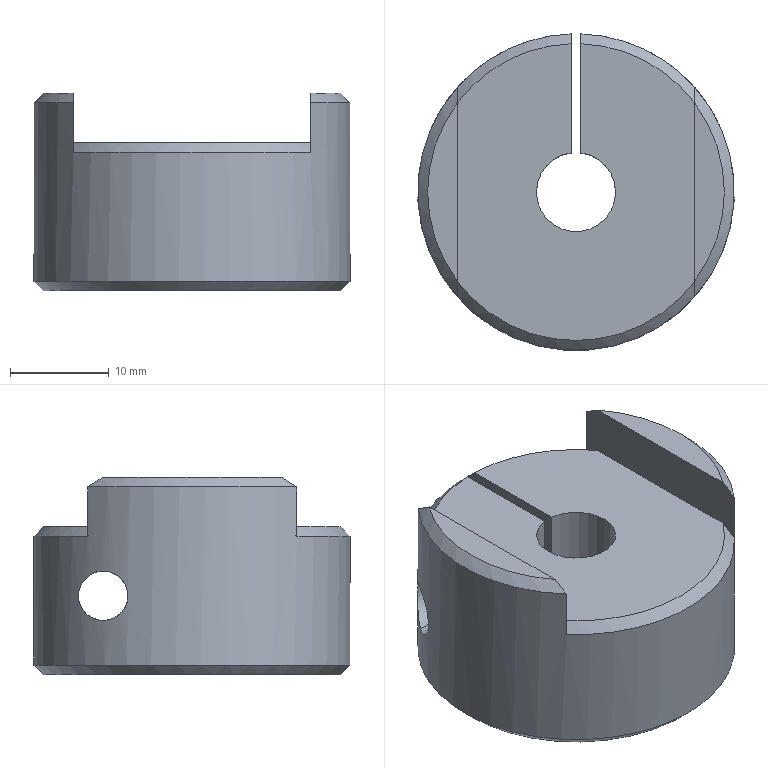Part | Creo | features CURVE 3, DATUM PLANE 3, CUT 2, CHAMFER 1, COORDINATE SYSTEM 1, PROTRUSION 1 | 1 solid | 20 faces | volume 11116 mm3 | plane 8 | cone 6 | cylinder 6 | commonest cylinder face diameters 5 x4 8 x1 32 x1